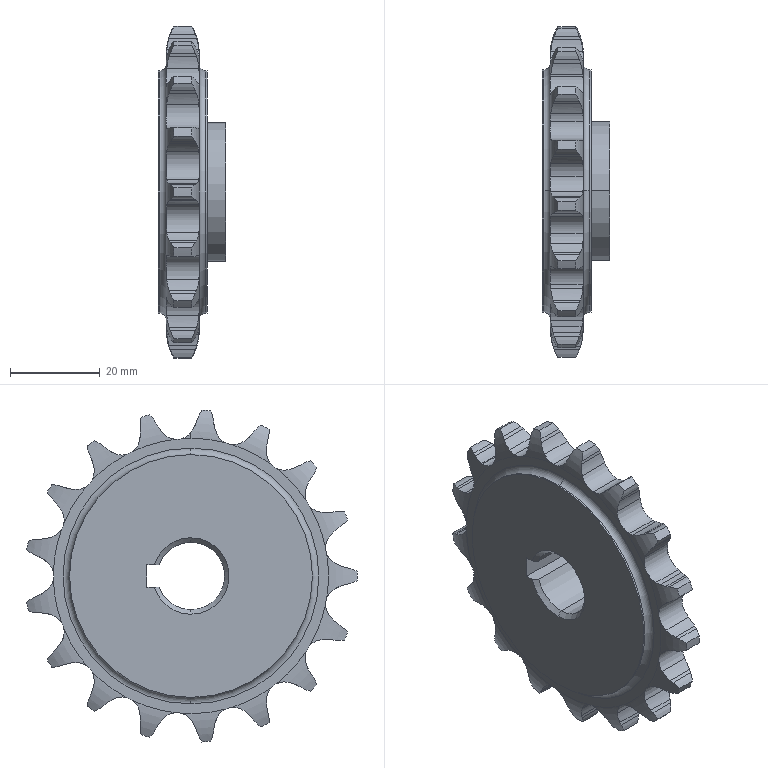Part | SolidWorks | features Chamfer 2, Cut 2, Revolution 2, CirPattern 1 | 1 solid | 206 faces | box 15 x 73.539 x 73.841 mm | volume 33361 mm3 | cylinder 118 | plane 42 | torus 40 | cone 6 | commonest cylinder face diameters 11.57 x35 20.732 x35 8.06 x22 74 x17 54 x4 15 x3